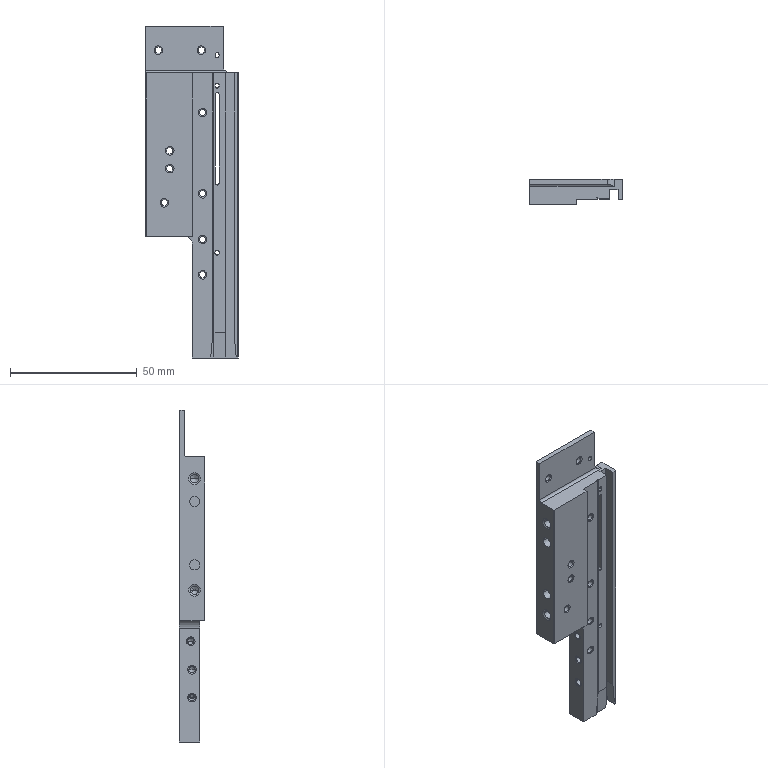Part | NX | 1 solid | 121 faces | box 36.55 x 10 x 131 mm | volume 26236 mm3 | cylinder 47 | cone 38 | plane 36 | commonest cylinder face diameters 2.5 x25 1.5 x9 3.3 x4 4 x4 1.8 x2 6 x2